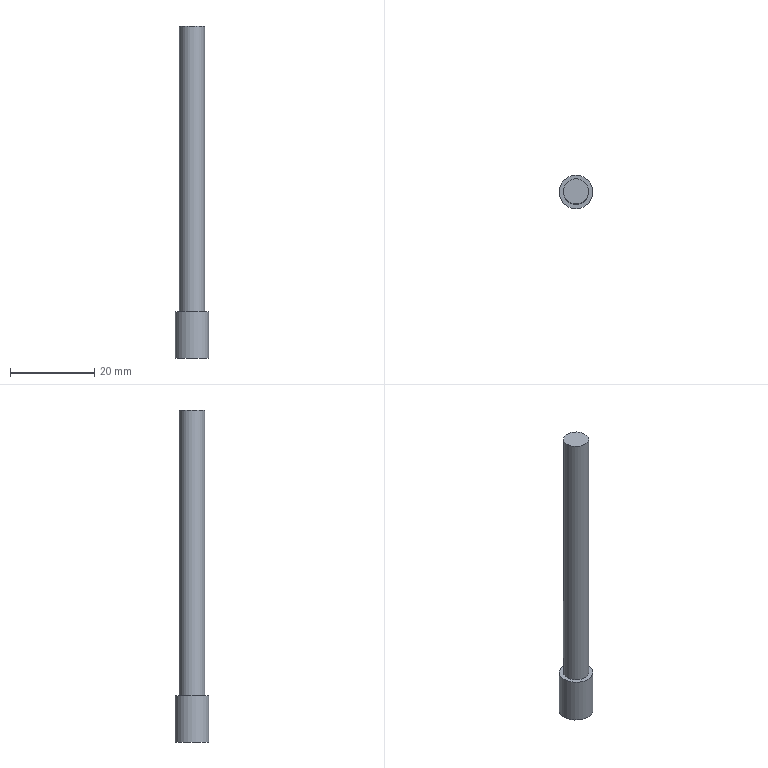Part | NX | features solid 2 | 1 solid | 5 faces | box 8 x 8 x 79 mm | volume 2476 mm3 | plane 3 | cylinder 2 | commonest cylinder face diameters 6 x1 8 x1
STEP:
#1=CARTESIAN_POINT('',(-93.,72.,29.));
#2=VERTEX_POINT('',#1);
#3=CARTESIAN_POINT('',(-90.,72.,29.));
#4=DIRECTION('',(0.,0.,1.));
#5=DIRECTION('',(-1.,0.,0.));
#6=AXIS2_PLACEMENT_3D('',#3,#4,#5);
#7=CIRCLE('',#6,3.);
#8=EDGE_CURVE('',#2,#2,#7,.F.);
#9=ORIENTED_EDGE('',*,*,#8,.T.);
#10=EDGE_LOOP('',(#9));
#11=FACE_BOUND('',#10,.T.);
#12=CARTESIAN_POINT('',(-87.,72.,-39.));
#13=VERTEX_POINT('',#12);
#14=CARTESIAN_POINT('',(-90.,72.,-39.));
#15=DIRECTION('',(0.,0.,1.));
#16=DIRECTION('',(1.,0.,0.));
#17=AXIS2_PLACEMENT_3D('',#14,#15,#16);
#18=CIRCLE('',#17,3.);
#19=EDGE_CURVE('',#13,#13,#18,.F.);
#20=ORIENTED_EDGE('',*,*,#19,.F.);
#21=EDGE_LOOP('',(#20));
#22=FACE_BOUND('',#21,.T.);
#23=CARTESIAN_POINT('',(-90.,72.,-35.));
#24=DIRECTION('',(0.,0.,1.));
#25=DIRECTION('',(-1.,0.,0.));
#26=AXIS2_PLACEMENT_3D('',#23,#24,#25);
#27=CYLINDRICAL_SURFACE('',#26,3.);
#28=ADVANCED_FACE('',(#11,#22),#27,.T.);
#29=ORIENTED_EDGE('',*,*,#8,.F.);
#30=EDGE_LOOP('',(#29));
#31=FACE_BOUND('',#30,.T.);
#32=CARTESIAN_POINT('',(-90.,72.,29.));
#33=DIRECTION('',(0.,0.,1.));
#34=DIRECTION('',(-1.,0.,0.));
#35=AXIS2_PLACEMENT_3D('',#32,#33,#34);
#36=PLANE('',#35);
#37=ADVANCED_FACE('',(#31),#36,.T.);
#38=CARTESIAN_POINT('',(-86.,72.,-39.));
#39=VERTEX_POINT('',#38);
#40=CARTESIAN_POINT('',(-90.,72.,-39.));
#41=DIRECTION('',(0.,0.,1.));
#42=DIRECTION('',(1.,0.,0.));
#43=AXIS2_PLACEMENT_3D('',#40,#41,#42);
#44=CIRCLE('',#43,4.);
#45=EDGE_CURVE('',#39,#39,#44,.T.);
#46=ORIENTED_EDGE('',*,*,#45,.F.);
#47=EDGE_LOOP('',(#46));
#48=FACE_BOUND('',#47,.T.);
#49=CARTESIAN_POINT('',(-86.,72.,-50.));
#50=VERTEX_POINT('',#49);
#51=CARTESIAN_POINT('',(-90.,72.,-50.));
#52=DIRECTION('',(0.,0.,1.));
#53=DIRECTION('',(1.,0.,0.));
#54=AXIS2_PLACEMENT_3D('',#51,#52,#53);
#55=CIRCLE('',#54,4.);
#56=EDGE_CURVE('',#50,#50,#55,.T.);
#57=ORIENTED_EDGE('',*,*,#56,.T.);
#58=EDGE_LOOP('',(#57));
#59=FACE_BOUND('',#58,.T.);
#60=CARTESIAN_POINT('',(-90.,72.,-38.));
#61=DIRECTION('',(0.,0.,-1.));
#62=DIRECTION('',(1.,0.,0.));
#63=AXIS2_PLACEMENT_3D('',#60,#61,#62);
#64=CYLINDRICAL_SURFACE('',#63,4.);
#65=ADVANCED_FACE('',(#48,#59),#64,.T.);
#66=ORIENTED_EDGE('',*,*,#19,.T.);
#67=EDGE_LOOP('',(#66));
#68=FACE_BOUND('',#67,.T.);
#69=ORIENTED_EDGE('',*,*,#45,.T.);
#70=EDGE_LOOP('',(#69));
#71=FACE_BOUND('',#70,.T.);
#72=CARTESIAN_POINT('',(-90.,72.,-39.));
#73=DIRECTION('',(0.,0.,-1.));
#74=DIRECTION('',(1.,0.,0.));
#75=AXIS2_PLACEMENT_3D('',#72,#73,#74);
#76=PLANE('',#75);
#77=ADVANCED_FACE('',(#68,#71),#76,.F.);
#78=ORIENTED_EDGE('',*,*,#56,.F.);
#79=EDGE_LOOP('',(#78));
#80=FACE_BOUND('',#79,.T.);
#81=CARTESIAN_POINT('',(-8.802,-46.836,-50.));
#82=DIRECTION('',(0.,0.,1.));
#83=DIRECTION('',(1.,0.,0.));
#84=AXIS2_PLACEMENT_3D('',#81,#82,#83);
#85=PLANE('',#84);
#86=ADVANCED_FACE('',(#80),#85,.F.);
#87=CLOSED_SHELL('',(#28,#37,#65,#77,#86));
#88=MANIFOLD_SOLID_BREP('',#87);
#89=(LENGTH_UNIT()NAMED_UNIT(*)SI_UNIT(.MILLI.,.METRE.));
#90=UNCERTAINTY_MEASURE_WITH_UNIT(LENGTH_MEASURE(0.00001),#89,'','');
#91=(NAMED_UNIT(*)PLANE_ANGLE_UNIT()SI_UNIT($,.RADIAN.));
#92=(NAMED_UNIT(*)SI_UNIT($,.STERADIAN.)SOLID_ANGLE_UNIT());
#93=(GEOMETRIC_REPRESENTATION_CONTEXT(3)GLOBAL_UNCERTAINTY_ASSIGNED_CONTEXT((#90))GLOBAL_UNIT_ASSIGNED_CONTEXT((#89,#91,#92))REPRESENTATION_CONTEXT('',''));
#94=ADVANCED_BREP_SHAPE_REPRESENTATION('',(#88),#93);